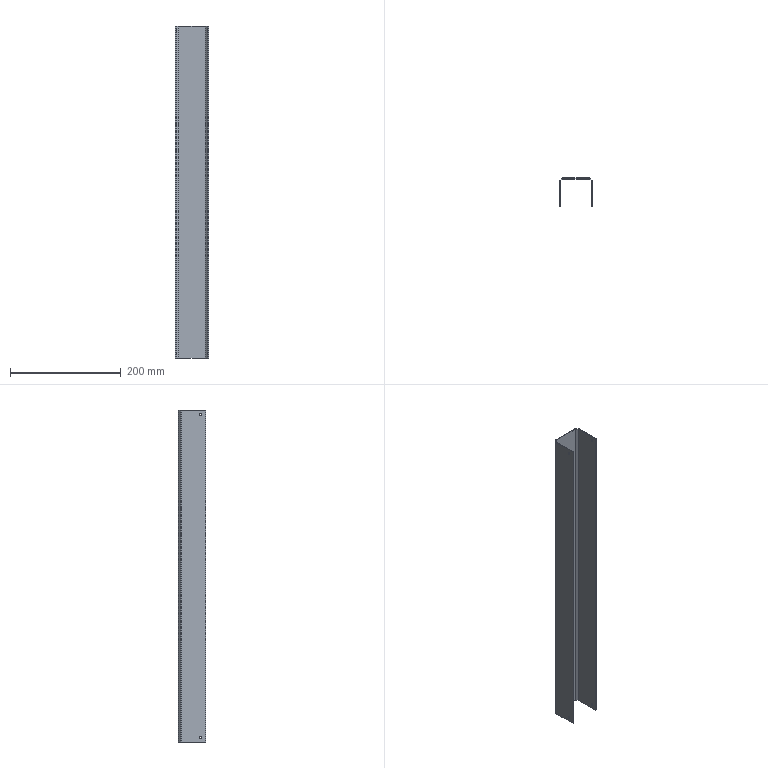Part | STEP file | Push-film group guard box SGN-3-06 | 1 solid | 46 faces | box 60 x 50 x 600 mm | volume 136056 mm3 | plane 30 | cylinder 16 | commonest cylinder face diameters 4.3 x8 3 x4 6 x4